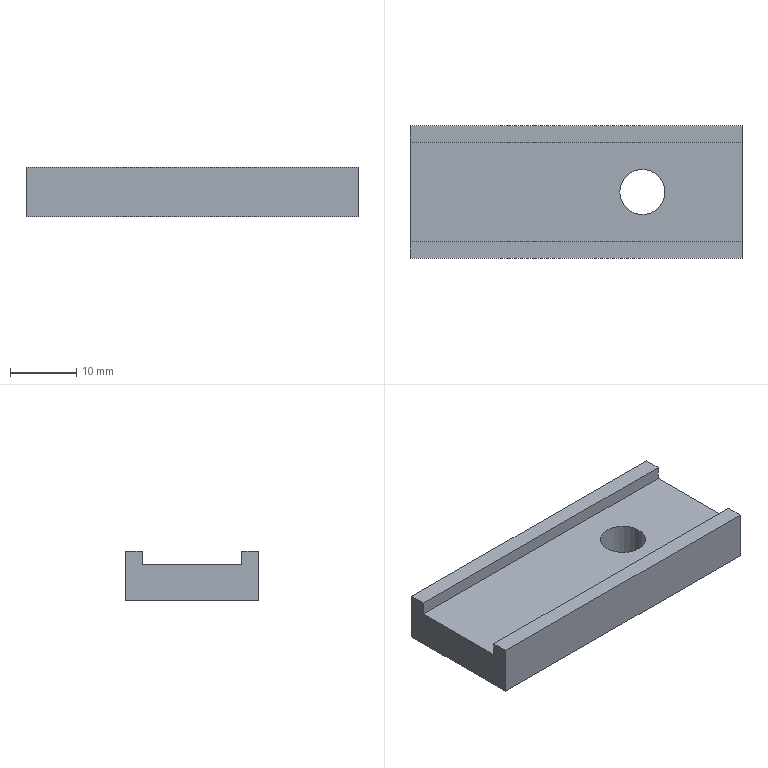Part | STEP file | Driven lead screw fixed block QY-1-17 | 1 solid | 12 faces | box 50 x 20 x 7.5 mm | volume 5800 mm3 | plane 10 | cylinder 2 | commonest cylinder face diameters 6.8 x2
STEP:
#1=CARTESIAN_POINT('',(0.,0.,0.));
#2=DIRECTION('',(0.,0.,1.));
#3=DIRECTION('',(1.,0.,0.));
#4=AXIS2_PLACEMENT_3D('',#1,#2,#3);
#5=CARTESIAN_POINT('',(13.4,0.,0.));
#6=VERTEX_POINT('',#5);
#7=CARTESIAN_POINT('',(13.4,0.,5.5));
#8=VERTEX_POINT('',#7);
#9=CARTESIAN_POINT('',(13.4,0.,5.5));
#10=DIRECTION('',(0.,0.,1.));
#11=VECTOR('',#10,1.);
#12=LINE('',#9,#11);
#13=CARTESIAN_POINT('',(10.,0.,5.5));
#14=DIRECTION('',(0.,0.,1.));
#15=DIRECTION('',(1.,0.,0.));
#16=AXIS2_PLACEMENT_3D('',#13,#14,#15);
#17=CYLINDRICAL_SURFACE('',#16,3.4);
#18=CARTESIAN_POINT('',(6.283,0.));
#19=DIRECTION('',(0.,1.));
#20=VECTOR('',#19,1.);
#21=LINE('',#18,#20);
#22=(GEOMETRIC_REPRESENTATION_CONTEXT(2)PARAMETRIC_REPRESENTATION_CONTEXT()REPRESENTATION_CONTEXT('',''));
#23=DEFINITIONAL_REPRESENTATION('',(#21),#22);
#24=PCURVE('',#17,#23);
#25=CARTESIAN_POINT('',(10.,0.,5.5));
#26=DIRECTION('',(0.,0.,1.));
#27=DIRECTION('',(1.,0.,0.));
#28=AXIS2_PLACEMENT_3D('',#25,#26,#27);
#29=CYLINDRICAL_SURFACE('',#28,3.4);
#30=CARTESIAN_POINT('',(0.,0.));
#31=DIRECTION('',(0.,1.));
#32=VECTOR('',#31,1.);
#33=LINE('',#30,#32);
#34=(GEOMETRIC_REPRESENTATION_CONTEXT(2)PARAMETRIC_REPRESENTATION_CONTEXT()REPRESENTATION_CONTEXT('',''));
#35=DEFINITIONAL_REPRESENTATION('',(#33),#34);
#36=PCURVE('',#29,#35);
#37=SURFACE_CURVE('',#12,(#24,#36),.PCURVE_S1.);
#38=EDGE_CURVE('',#6,#8,#37,.T.);
#39=ORIENTED_EDGE('',*,*,#38,.T.);
#40=CARTESIAN_POINT('',(6.6,0.,5.5));
#41=VERTEX_POINT('',#40);
#42=CARTESIAN_POINT('',(10.,0.,5.5));
#43=DIRECTION('',(0.,0.,1.));
#44=DIRECTION('',(1.,0.,0.));
#45=AXIS2_PLACEMENT_3D('',#42,#43,#44);
#46=CIRCLE('',#45,3.4);
#47=CARTESIAN_POINT('',(0.,0.));
#48=DIRECTION('',(1.,0.));
#49=VECTOR('',#48,1.);
#50=LINE('',#47,#49);
#51=(GEOMETRIC_REPRESENTATION_CONTEXT(2)PARAMETRIC_REPRESENTATION_CONTEXT()REPRESENTATION_CONTEXT('',''));
#52=DEFINITIONAL_REPRESENTATION('',(#50),#51);
#53=PCURVE('',#17,#52);
#54=CARTESIAN_POINT('',(0.,0.,5.5));
#55=DIRECTION('',(0.,0.,-1.));
#56=DIRECTION('',(-1.,0.,0.));
#57=AXIS2_PLACEMENT_3D('',#54,#55,#56);
#58=PLANE('',#57);
#59=CARTESIAN_POINT('',(-13.4,0.));
#60=CARTESIAN_POINT('',(-13.4,5.889));
#61=CARTESIAN_POINT('',(-8.3,2.944));
#62=CARTESIAN_POINT('',(-3.2,0.));
#63=CARTESIAN_POINT('',(-8.3,-2.944));
#64=CARTESIAN_POINT('',(-13.4,-5.889));
#65=CARTESIAN_POINT('',(-13.4,0.));
#66=(BOUNDED_CURVE()B_SPLINE_CURVE(2,(#59,#60,#61,#62,#63,#64,#65),.UNSPECIFIED.,.T.,.F.)B_SPLINE_CURVE_WITH_KNOTS((1,2,2,2,2,1),(-2.094,0.,2.094,4.189,6.283,8.378),.UNSPECIFIED.)CURVE()GEOMETRIC_REPRESENTATION_ITEM()RATIONAL_B_SPLINE_CURVE((1.,0.5,1.,0.5,1.,0.5,1.))REPRESENTATION_ITEM(''));
#67=(GEOMETRIC_REPRESENTATION_CONTEXT(2)PARAMETRIC_REPRESENTATION_CONTEXT()REPRESENTATION_CONTEXT('',''));
#68=DEFINITIONAL_REPRESENTATION('',(#66),#67);
#69=PCURVE('',#58,#68);
#70=SURFACE_CURVE('',#46,(#53,#69),.PCURVE_S1.);
#71=EDGE_CURVE('',#41,#8,#70,.T.);
#72=ORIENTED_EDGE('',*,*,#71,.F.);
#73=CARTESIAN_POINT('',(6.6,0.,0.));
#74=VERTEX_POINT('',#73);
#75=CARTESIAN_POINT('',(6.6,0.,5.5));
#76=DIRECTION('',(0.,0.,1.));
#77=VECTOR('',#76,1.);
#78=LINE('',#75,#77);
#79=CARTESIAN_POINT('',(3.142,0.));
#80=DIRECTION('',(0.,1.));
#81=VECTOR('',#80,1.);
#82=LINE('',#79,#81);
#83=(GEOMETRIC_REPRESENTATION_CONTEXT(2)PARAMETRIC_REPRESENTATION_CONTEXT()REPRESENTATION_CONTEXT('',''));
#84=DEFINITIONAL_REPRESENTATION('',(#82),#83);
#85=PCURVE('',#17,#84);
#86=CARTESIAN_POINT('',(3.142,0.));
#87=DIRECTION('',(0.,1.));
#88=VECTOR('',#87,1.);
#89=LINE('',#86,#88);
#90=(GEOMETRIC_REPRESENTATION_CONTEXT(2)PARAMETRIC_REPRESENTATION_CONTEXT()REPRESENTATION_CONTEXT('',''));
#91=DEFINITIONAL_REPRESENTATION('',(#89),#90);
#92=PCURVE('',#29,#91);
#93=SURFACE_CURVE('',#78,(#85,#92),.PCURVE_S1.);
#94=EDGE_CURVE('',#74,#41,#93,.T.);
#95=ORIENTED_EDGE('',*,*,#94,.F.);
#96=CARTESIAN_POINT('',(10.,0.,0.));
#97=DIRECTION('',(0.,0.,1.));
#98=DIRECTION('',(1.,0.,0.));
#99=AXIS2_PLACEMENT_3D('',#96,#97,#98);
#100=CIRCLE('',#99,3.4);
#101=CARTESIAN_POINT('',(0.,-5.5));
#102=DIRECTION('',(1.,0.));
#103=VECTOR('',#102,1.);
#104=LINE('',#101,#103);
#105=(GEOMETRIC_REPRESENTATION_CONTEXT(2)PARAMETRIC_REPRESENTATION_CONTEXT()REPRESENTATION_CONTEXT('',''));
#106=DEFINITIONAL_REPRESENTATION('',(#104),#105);
#107=PCURVE('',#17,#106);
#108=CARTESIAN_POINT('',(0.,0.,0.));
#109=DIRECTION('',(0.,0.,1.));
#110=DIRECTION('',(1.,0.,0.));
#111=AXIS2_PLACEMENT_3D('',#108,#109,#110);
#112=PLANE('',#111);
#113=CARTESIAN_POINT('',(10.,0.));
#114=DIRECTION('',(1.,0.));
#115=AXIS2_PLACEMENT_2D('',#113,#114);
#116=CIRCLE('',#115,3.4);
#117=(GEOMETRIC_REPRESENTATION_CONTEXT(2)PARAMETRIC_REPRESENTATION_CONTEXT()REPRESENTATION_CONTEXT('',''));
#118=DEFINITIONAL_REPRESENTATION('',(#116),#117);
#119=PCURVE('',#112,#118);
#120=SURFACE_CURVE('',#100,(#107,#119),.PCURVE_S1.);
#121=EDGE_CURVE('',#74,#6,#120,.T.);
#122=ORIENTED_EDGE('',*,*,#121,.T.);
#123=EDGE_LOOP('',(#39,#72,#95,#122));
#124=FACE_BOUND('',#123,.F.);
#125=ADVANCED_FACE('',(#124),#17,.F.);
#126=CARTESIAN_POINT('',(-25.,-7.5,7.5));
#127=VERTEX_POINT('',#126);
#128=CARTESIAN_POINT('',(25.,-7.5,7.5));
#129=VERTEX_POINT('',#128);
#130=CARTESIAN_POINT('',(0.,-7.5,7.5));
#131=DIRECTION('',(1.,0.,0.));
#132=VECTOR('',#131,1.);
#133=LINE('',#130,#132);
#134=CARTESIAN_POINT('',(0.,0.,7.5));
#135=DIRECTION('',(0.,0.,1.));
#136=DIRECTION('',(1.,0.,0.));
#137=AXIS2_PLACEMENT_3D('',#134,#135,#136);
#138=PLANE('',#137);
#139=CARTESIAN_POINT('',(0.,-7.5));
#140=DIRECTION('',(1.,0.));
#141=VECTOR('',#140,1.);
#142=LINE('',#139,#141);
#143=(GEOMETRIC_REPRESENTATION_CONTEXT(2)PARAMETRIC_REPRESENTATION_CONTEXT()REPRESENTATION_CONTEXT('',''));
#144=DEFINITIONAL_REPRESENTATION('',(#142),#143);
#145=PCURVE('',#138,#144);
#146=CARTESIAN_POINT('',(-35.049,-7.5,5.5));
#147=DIRECTION('',(0.,-1.,0.));
#148=DIRECTION('',(0.,0.,-1.));
#149=AXIS2_PLACEMENT_3D('',#146,#147,#148);
#150=PLANE('',#149);
#151=CARTESIAN_POINT('',(-2.,35.049));
#152=DIRECTION('',(0.,1.));
#153=VECTOR('',#152,1.);
#154=LINE('',#151,#153);
#155=(GEOMETRIC_REPRESENTATION_CONTEXT(2)PARAMETRIC_REPRESENTATION_CONTEXT()REPRESENTATION_CONTEXT('',''));
#156=DEFINITIONAL_REPRESENTATION('',(#154),#155);
#157=PCURVE('',#150,#156);
#158=SURFACE_CURVE('',#133,(#145,#157),.PCURVE_S1.);
#159=EDGE_CURVE('',#127,#129,#158,.T.);
#160=ORIENTED_EDGE('',*,*,#159,.F.);
#161=CARTESIAN_POINT('',(-25.,-10.,7.5));
#162=VERTEX_POINT('',#161);
#163=CARTESIAN_POINT('',(-25.,10.,7.5));
#164=DIRECTION('',(0.,-1.,0.));
#165=VECTOR('',#164,1.);
#166=LINE('',#163,#165);
#167=CARTESIAN_POINT('',(-25.,10.));
#168=DIRECTION('',(0.,-1.));
#169=VECTOR('',#168,1.);
#170=LINE('',#167,#169);
#171=(GEOMETRIC_REPRESENTATION_CONTEXT(2)PARAMETRIC_REPRESENTATION_CONTEXT()REPRESENTATION_CONTEXT('',''));
#172=DEFINITIONAL_REPRESENTATION('',(#170),#171);
#173=PCURVE('',#138,#172);
#174=CARTESIAN_POINT('',(-25.,10.,7.5));
#175=DIRECTION('',(1.,0.,0.));
#176=DIRECTION('',(0.,0.,-1.));
#177=AXIS2_PLACEMENT_3D('',#174,#175,#176);
#178=PLANE('',#177);
#179=CARTESIAN_POINT('',(0.,0.));
#180=DIRECTION('',(0.,-1.));
#181=VECTOR('',#180,1.);
#182=LINE('',#179,#181);
#183=(GEOMETRIC_REPRESENTATION_CONTEXT(2)PARAMETRIC_REPRESENTATION_CONTEXT()REPRESENTATION_CONTEXT('',''));
#184=DEFINITIONAL_REPRESENTATION('',(#182),#183);
#185=PCURVE('',#178,#184);
#186=SURFACE_CURVE('',#166,(#173,#185),.PCURVE_S1.);
#187=EDGE_CURVE('',#127,#162,#186,.T.);
#188=ORIENTED_EDGE('',*,*,#187,.T.);
#189=CARTESIAN_POINT('',(25.,-10.,7.5));
#190=VERTEX_POINT('',#189);
#191=CARTESIAN_POINT('',(-25.,-10.,7.5));
#192=DIRECTION('',(1.,0.,0.));
#193=VECTOR('',#192,1.);
#194=LINE('',#191,#193);
#195=CARTESIAN_POINT('',(-25.,-10.));
#196=DIRECTION('',(1.,0.));
#197=VECTOR('',#196,1.);
#198=LINE('',#195,#197);
#199=(GEOMETRIC_REPRESENTATION_CONTEXT(2)PARAMETRIC_REPRESENTATION_CONTEXT()REPRESENTATION_CONTEXT('',''));
#200=DEFINITIONAL_REPRESENTATION('',(#198),#199);
#201=PCURVE('',#138,#200);
#202=CARTESIAN_POINT('',(-25.,-10.,7.5));
#203=DIRECTION('',(0.,1.,0.));
#204=DIRECTION('',(0.,0.,1.));
#205=AXIS2_PLACEMENT_3D('',#202,#203,#204);
#206=PLANE('',#205);
#207=CARTESIAN_POINT('',(0.,0.));
#208=DIRECTION('',(0.,1.));
#209=VECTOR('',#208,1.);
#210=LINE('',#207,#209);
#211=(GEOMETRIC_REPRESENTATION_CONTEXT(2)PARAMETRIC_REPRESENTATION_CONTEXT()REPRESENTATION_CONTEXT('',''));
#212=DEFINITIONAL_REPRESENTATION('',(#210),#211);
#213=PCURVE('',#206,#212);
#214=SURFACE_CURVE('',#194,(#201,#213),.PCURVE_S1.);
#215=EDGE_CURVE('',#162,#190,#214,.T.);
#216=ORIENTED_EDGE('',*,*,#215,.T.);
#217=CARTESIAN_POINT('',(25.,10.,7.5));
#218=DIRECTION('',(0.,1.,0.));
#219=VECTOR('',#218,1.);
#220=LINE('',#217,#219);
#221=CARTESIAN_POINT('',(25.,10.));
#222=DIRECTION('',(0.,1.));
#223=VECTOR('',#222,1.);
#224=LINE('',#221,#223);
#225=(GEOMETRIC_REPRESENTATION_CONTEXT(2)PARAMETRIC_REPRESENTATION_CONTEXT()REPRESENTATION_CONTEXT('',''));
#226=DEFINITIONAL_REPRESENTATION('',(#224),#225);
#227=PCURVE('',#138,#226);
#228=CARTESIAN_POINT('',(25.,10.,7.5));
#229=DIRECTION('',(-1.,0.,0.));
#230=DIRECTION('',(0.,-1.,0.));
#231=AXIS2_PLACEMENT_3D('',#228,#229,#230);
#232=PLANE('',#231);
#233=CARTESIAN_POINT('',(0.,0.));
#234=DIRECTION('',(-1.,0.));
#235=VECTOR('',#234,1.);
#236=LINE('',#233,#235);
#237=(GEOMETRIC_REPRESENTATION_CONTEXT(2)PARAMETRIC_REPRESENTATION_CONTEXT()REPRESENTATION_CONTEXT('',''));
#238=DEFINITIONAL_REPRESENTATION('',(#236),#237);
#239=PCURVE('',#232,#238);
#240=SURFACE_CURVE('',#220,(#227,#239),.PCURVE_S1.);
#241=EDGE_CURVE('',#190,#129,#240,.T.);
#242=ORIENTED_EDGE('',*,*,#241,.T.);
#243=EDGE_LOOP('',(#160,#188,#216,#242));
#244=FACE_BOUND('',#243,.T.);
#245=ADVANCED_FACE('',(#244),#138,.T.);
#246=CARTESIAN_POINT('',(25.,7.5,5.5));
#247=VERTEX_POINT('',#246);
#248=CARTESIAN_POINT('',(25.,-7.5,5.5));
#249=VERTEX_POINT('',#248);
#250=CARTESIAN_POINT('',(25.,10.,5.5));
#251=DIRECTION('',(0.,-1.,0.));
#252=VECTOR('',#251,1.);
#253=LINE('',#250,#252);
#254=CARTESIAN_POINT('',(0.,-2.));
#255=DIRECTION('',(1.,0.));
#256=VECTOR('',#255,1.);
#257=LINE('',#254,#256);
#258=(GEOMETRIC_REPRESENTATION_CONTEXT(2)PARAMETRIC_REPRESENTATION_CONTEXT()REPRESENTATION_CONTEXT('',''));
#259=DEFINITIONAL_REPRESENTATION('',(#257),#258);
#260=PCURVE('',#232,#259);
#261=CARTESIAN_POINT('',(-25.,10.));
#262=DIRECTION('',(0.,-1.));
#263=VECTOR('',#262,1.);
#264=LINE('',#261,#263);
#265=(GEOMETRIC_REPRESENTATION_CONTEXT(2)PARAMETRIC_REPRESENTATION_CONTEXT()REPRESENTATION_CONTEXT('',''));
#266=DEFINITIONAL_REPRESENTATION('',(#264),#265);
#267=PCURVE('',#58,#266);
#268=SURFACE_CURVE('',#253,(#260,#267),.PCURVE_S1.);
#269=EDGE_CURVE('',#247,#249,#268,.T.);
#270=ORIENTED_EDGE('',*,*,#269,.T.);
#271=CARTESIAN_POINT('',(25.,-7.5,7.5));
#272=DIRECTION('',(0.,0.,1.));
#273=VECTOR('',#272,1.);
#274=LINE('',#271,#273);
#275=CARTESIAN_POINT('',(17.5,0.));
#276=DIRECTION('',(0.,1.));
#277=VECTOR('',#276,1.);
#278=LINE('',#275,#277);
#279=(GEOMETRIC_REPRESENTATION_CONTEXT(2)PARAMETRIC_REPRESENTATION_CONTEXT()REPRESENTATION_CONTEXT('',''));
#280=DEFINITIONAL_REPRESENTATION('',(#278),#279);
#281=PCURVE('',#232,#280);
#282=CARTESIAN_POINT('',(-2.,60.049));
#283=DIRECTION('',(-1.,0.));
#284=VECTOR('',#283,1.);
#285=LINE('',#282,#284);
#286=(GEOMETRIC_REPRESENTATION_CONTEXT(2)PARAMETRIC_REPRESENTATION_CONTEXT()REPRESENTATION_CONTEXT('',''));
#287=DEFINITIONAL_REPRESENTATION('',(#285),#286);
#288=PCURVE('',#150,#287);
#289=SURFACE_CURVE('',#274,(#281,#288),.PCURVE_S1.);
#290=EDGE_CURVE('',#249,#129,#289,.T.);
#291=ORIENTED_EDGE('',*,*,#290,.T.);
#292=ORIENTED_EDGE('',*,*,#241,.F.);
#293=CARTESIAN_POINT('',(25.,-10.,0.));
#294=VERTEX_POINT('',#293);
#295=CARTESIAN_POINT('',(25.,-10.,7.5));
#296=DIRECTION('',(0.,0.,-1.));
#297=VECTOR('',#296,1.);
#298=LINE('',#295,#297);
#299=CARTESIAN_POINT('',(20.,0.));
#300=DIRECTION('',(0.,-1.));
#301=VECTOR('',#300,1.);
#302=LINE('',#299,#301);
#303=(GEOMETRIC_REPRESENTATION_CONTEXT(2)PARAMETRIC_REPRESENTATION_CONTEXT()REPRESENTATION_CONTEXT('',''));
#304=DEFINITIONAL_REPRESENTATION('',(#302),#303);
#305=PCURVE('',#232,#304);
#306=CARTESIAN_POINT('',(0.,50.));
#307=DIRECTION('',(-1.,0.));
#308=VECTOR('',#307,1.);
#309=LINE('',#306,#308);
#310=(GEOMETRIC_REPRESENTATION_CONTEXT(2)PARAMETRIC_REPRESENTATION_CONTEXT()REPRESENTATION_CONTEXT('',''));
#311=DEFINITIONAL_REPRESENTATION('',(#309),#310);
#312=PCURVE('',#206,#311);
#313=SURFACE_CURVE('',#298,(#305,#312),.PCURVE_S1.);
#314=EDGE_CURVE('',#190,#294,#313,.T.);
#315=ORIENTED_EDGE('',*,*,#314,.T.);
#316=CARTESIAN_POINT('',(25.,10.,0.));
#317=VERTEX_POINT('',#316);
#318=CARTESIAN_POINT('',(25.,10.,0.));
#319=DIRECTION('',(0.,1.,0.));
#320=VECTOR('',#319,1.);
#321=LINE('',#318,#320);
#322=CARTESIAN_POINT('',(0.,-7.5));
#323=DIRECTION('',(-1.,0.));
#324=VECTOR('',#323,1.);
#325=LINE('',#322,#324);
#326=(GEOMETRIC_REPRESENTATION_CONTEXT(2)PARAMETRIC_REPRESENTATION_CONTEXT()REPRESENTATION_CONTEXT('',''));
#327=DEFINITIONAL_REPRESENTATION('',(#325),#326);
#328=PCURVE('',#232,#327);
#329=CARTESIAN_POINT('',(25.,10.));
#330=DIRECTION('',(0.,1.));
#331=VECTOR('',#330,1.);
#332=LINE('',#329,#331);
#333=(GEOMETRIC_REPRESENTATION_CONTEXT(2)PARAMETRIC_REPRESENTATION_CONTEXT()REPRESENTATION_CONTEXT('',''));
#334=DEFINITIONAL_REPRESENTATION('',(#332),#333);
#335=PCURVE('',#112,#334);
#336=SURFACE_CURVE('',#321,(#328,#335),.PCURVE_S1.);
#337=EDGE_CURVE('',#294,#317,#336,.T.);
#338=ORIENTED_EDGE('',*,*,#337,.T.);
#339=CARTESIAN_POINT('',(25.,10.,7.5));
#340=VERTEX_POINT('',#339);
#341=CARTESIAN_POINT('',(25.,10.,7.5));
#342=DIRECTION('',(0.,0.,-1.));
#343=VECTOR('',#342,1.);
#344=LINE('',#341,#343);
#345=CARTESIAN_POINT('',(0.,0.));
#346=DIRECTION('',(0.,-1.));
#347=VECTOR('',#346,1.);
#348=LINE('',#345,#347);
#349=(GEOMETRIC_REPRESENTATION_CONTEXT(2)PARAMETRIC_REPRESENTATION_CONTEXT()REPRESENTATION_CONTEXT('',''));
#350=DEFINITIONAL_REPRESENTATION('',(#348),#349);
#351=PCURVE('',#232,#350);
#352=CARTESIAN_POINT('',(-25.,10.,7.5));
#353=DIRECTION('',(0.,-1.,0.));
#354=DIRECTION('',(0.,0.,-1.));
#355=AXIS2_PLACEMENT_3D('',#352,#353,#354);
#356=PLANE('',#355);
#357=CARTESIAN_POINT('',(0.,50.));
#358=DIRECTION('',(1.,0.));
#359=VECTOR('',#358,1.);
#360=LINE('',#357,#359);
#361=(GEOMETRIC_REPRESENTATION_CONTEXT(2)PARAMETRIC_REPRESENTATION_CONTEXT()REPRESENTATION_CONTEXT('',''));
#362=DEFINITIONAL_REPRESENTATION('',(#360),#361);
#363=PCURVE('',#356,#362);
#364=SURFACE_CURVE('',#344,(#351,#363),.PCURVE_S1.);
#365=EDGE_CURVE('',#340,#317,#364,.T.);
#366=ORIENTED_EDGE('',*,*,#365,.F.);
#367=CARTESIAN_POINT('',(25.,7.5,7.5));
#368=VERTEX_POINT('',#367);
#369=CARTESIAN_POINT('',(25.,10.,7.5));
#370=DIRECTION('',(0.,1.,0.));
#371=VECTOR('',#370,1.);
#372=LINE('',#369,#371);
#373=CARTESIAN_POINT('',(0.,0.));
#374=DIRECTION('',(-1.,0.));
#375=VECTOR('',#374,1.);
#376=LINE('',#373,#375);
#377=(GEOMETRIC_REPRESENTATION_CONTEXT(2)PARAMETRIC_REPRESENTATION_CONTEXT()REPRESENTATION_CONTEXT('',''));
#378=DEFINITIONAL_REPRESENTATION('',(#376),#377);
#379=PCURVE('',#232,#378);
#380=CARTESIAN_POINT('',(0.,0.,7.5));
#381=DIRECTION('',(0.,0.,1.));
#382=DIRECTION('',(1.,0.,0.));
#383=AXIS2_PLACEMENT_3D('',#380,#381,#382);
#384=PLANE('',#383);
#385=CARTESIAN_POINT('',(25.,10.));
#386=DIRECTION('',(0.,1.));
#387=VECTOR('',#386,1.);
#388=LINE('',#385,#387);
#389=(GEOMETRIC_REPRESENTATION_CONTEXT(2)PARAMETRIC_REPRESENTATION_CONTEXT()REPRESENTATION_CONTEXT('',''));
#390=DEFINITIONAL_REPRESENTATION('',(#388),#389);
#391=PCURVE('',#384,#390);
#392=SURFACE_CURVE('',#372,(#379,#391),.PCURVE_S1.);
#393=EDGE_CURVE('',#368,#340,#392,.T.);
#394=ORIENTED_EDGE('',*,*,#393,.F.);
#395=CARTESIAN_POINT('',(25.,7.5,7.5));
#396=DIRECTION('',(0.,0.,-1.));
#397=VECTOR('',#396,1.);
#398=LINE('',#395,#397);
#399=CARTESIAN_POINT('',(2.5,0.));
#400=DIRECTION('',(0.,-1.));
#401=VECTOR('',#400,1.);
#402=LINE('',#399,#401);
#403=(GEOMETRIC_REPRESENTATION_CONTEXT(2)PARAMETRIC_REPRESENTATION_CONTEXT()REPRESENTATION_CONTEXT('',''));
#404=DEFINITIONAL_REPRESENTATION('',(#402),#403);
#405=PCURVE('',#232,#404);
#406=CARTESIAN_POINT('',(-35.049,7.5,5.5));
#407=DIRECTION('',(0.,1.,0.));
#408=DIRECTION('',(0.,0.,1.));
#409=AXIS2_PLACEMENT_3D('',#406,#407,#408);
#410=PLANE('',#409);
#411=CARTESIAN_POINT('',(2.,60.049));
#412=DIRECTION('',(-1.,0.));
#413=VECTOR('',#412,1.);
#414=LINE('',#411,#413);
#415=(GEOMETRIC_REPRESENTATION_CONTEXT(2)PARAMETRIC_REPRESENTATION_CONTEXT()REPRESENTATION_CONTEXT('',''));
#416=DEFINITIONAL_REPRESENTATION('',(#414),#415);
#417=PCURVE('',#410,#416);
#418=SURFACE_CURVE('',#398,(#405,#417),.PCURVE_S1.);
#419=EDGE_CURVE('',#368,#247,#418,.T.);
#420=ORIENTED_EDGE('',*,*,#419,.T.);
#421=EDGE_LOOP('',(#270,#291,#292,#315,#338,#366,#394,#420));
#422=FACE_BOUND('',#421,.T.);
#423=ADVANCED_FACE('',(#422),#232,.F.);
#424=CARTESIAN_POINT('',(-25.,10.,0.));
#425=VERTEX_POINT('',#424);
#426=CARTESIAN_POINT('',(-25.,10.,0.));
#427=DIRECTION('',(-1.,0.,0.));
#428=VECTOR('',#427,1.);
#429=LINE('',#426,#428);
#430=CARTESIAN_POINT('',(7.5,0.));
#431=DIRECTION('',(0.,-1.));
#432=VECTOR('',#431,1.);
#433=LINE('',#430,#432);
#434=(GEOMETRIC_REPRESENTATION_CONTEXT(2)PARAMETRIC_REPRESENTATION_CONTEXT()REPRESENTATION_CONTEXT('',''));
#435=DEFINITIONAL_REPRESENTATION('',(#433),#434);
#436=PCURVE('',#356,#435);
#437=CARTESIAN_POINT('',(-25.,10.));
#438=DIRECTION('',(-1.,0.));
#439=VECTOR('',#438,1.);
#440=LINE('',#437,#439);
#441=(GEOMETRIC_REPRESENTATION_CONTEXT(2)PARAMETRIC_REPRESENTATION_CONTEXT()REPRESENTATION_CONTEXT('',''));
#442=DEFINITIONAL_REPRESENTATION('',(#440),#441);
#443=PCURVE('',#112,#442);
#444=SURFACE_CURVE('',#429,(#436,#443),.PCURVE_S1.);
#445=EDGE_CURVE('',#317,#425,#444,.T.);
#446=ORIENTED_EDGE('',*,*,#445,.T.);
#447=CARTESIAN_POINT('',(-25.,10.,7.5));
#448=VERTEX_POINT('',#447);
#449=CARTESIAN_POINT('',(-25.,10.,7.5));
#450=DIRECTION('',(0.,0.,-1.));
#451=VECTOR('',#450,1.);
#452=LINE('',#449,#451);
#453=CARTESIAN_POINT('',(0.,0.));
#454=DIRECTION('',(1.,0.));
#455=VECTOR('',#454,1.);
#456=LINE('',#453,#455);
#457=(GEOMETRIC_REPRESENTATION_CONTEXT(2)PARAMETRIC_REPRESENTATION_CONTEXT()REPRESENTATION_CONTEXT('',''));
#458=DEFINITIONAL_REPRESENTATION('',(#456),#457);
#459=PCURVE('',#356,#458);
#460=CARTESIAN_POINT('',(0.,0.));
#461=DIRECTION('',(1.,0.));
#462=VECTOR('',#461,1.);
#463=LINE('',#460,#462);
#464=(GEOMETRIC_REPRESENTATION_CONTEXT(2)PARAMETRIC_REPRESENTATION_CONTEXT()REPRESENTATION_CONTEXT('',''));
#465=DEFINITIONAL_REPRESENTATION('',(#463),#464);
#466=PCURVE('',#178,#465);
#467=SURFACE_CURVE('',#452,(#459,#466),.PCURVE_S1.);
#468=EDGE_CURVE('',#448,#425,#467,.T.);
#469=ORIENTED_EDGE('',*,*,#468,.F.);
#470=CARTESIAN_POINT('',(-25.,10.,7.5));
#471=DIRECTION('',(-1.,0.,0.));
#472=VECTOR('',#471,1.);
#473=LINE('',#470,#472);
#474=CARTESIAN_POINT('',(0.,0.));
#475=DIRECTION('',(0.,-1.));
#476=VECTOR('',#475,1.);
#477=LINE('',#474,#476);
#478=(GEOMETRIC_REPRESENTATION_CONTEXT(2)PARAMETRIC_REPRESENTATION_CONTEXT()REPRESENTATION_CONTEXT('',''));
#479=DEFINITIONAL_REPRESENTATION('',(#477),#478);
#480=PCURVE('',#356,#479);
#481=CARTESIAN_POINT('',(-25.,10.));
#482=DIRECTION('',(-1.,0.));
#483=VECTOR('',#482,1.);
#484=LINE('',#481,#483);
#485=(GEOMETRIC_REPRESENTATION_CONTEXT(2)PARAMETRIC_REPRESENTATION_CONTEXT()REPRESENTATION_CONTEXT('',''));
#486=DEFINITIONAL_REPRESENTATION('',(#484),#485);
#487=PCURVE('',#384,#486);
#488=SURFACE_CURVE('',#473,(#480,#487),.PCURVE_S1.);
#489=EDGE_CURVE('',#340,#448,#488,.T.);
#490=ORIENTED_EDGE('',*,*,#489,.F.);
#491=ORIENTED_EDGE('',*,*,#365,.T.);
#492=EDGE_LOOP('',(#446,#469,#490,#491));
#493=FACE_BOUND('',#492,.T.);
#494=ADVANCED_FACE('',(#493),#356,.F.);
#495=ORIENTED_EDGE('',*,*,#187,.F.);
#496=CARTESIAN_POINT('',(-25.,-7.5,5.5));
#497=VERTEX_POINT('',#496);
#498=CARTESIAN_POINT('',(-25.,-7.5,7.5));
#499=DIRECTION('',(0.,0.,-1.));
#500=VECTOR('',#499,1.);
#501=LINE('',#498,#500);
#502=CARTESIAN_POINT('',(0.,-17.5));
#503=DIRECTION('',(1.,0.));
#504=VECTOR('',#503,1.);
#505=LINE('',#502,#504);
#506=(GEOMETRIC_REPRESENTATION_CONTEXT(2)PARAMETRIC_REPRESENTATION_CONTEXT()REPRESENTATION_CONTEXT('',''));
#507=DEFINITIONAL_REPRESENTATION('',(#505),#506);
#508=PCURVE('',#178,#507);
#509=CARTESIAN_POINT('',(-2.,10.049));
#510=DIRECTION('',(1.,0.));
#511=VECTOR('',#510,1.);
#512=LINE('',#509,#511);
#513=(GEOMETRIC_REPRESENTATION_CONTEXT(2)PARAMETRIC_REPRESENTATION_CONTEXT()REPRESENTATION_CONTEXT('',''));
#514=DEFINITIONAL_REPRESENTATION('',(#512),#513);
#515=PCURVE('',#150,#514);
#516=SURFACE_CURVE('',#501,(#508,#515),.PCURVE_S1.);
#517=EDGE_CURVE('',#127,#497,#516,.T.);
#518=ORIENTED_EDGE('',*,*,#517,.T.);
#519=CARTESIAN_POINT('',(-25.,7.5,5.5));
#520=VERTEX_POINT('',#519);
#521=CARTESIAN_POINT('',(-25.,10.,5.5));
#522=DIRECTION('',(0.,1.,0.));
#523=VECTOR('',#522,1.);
#524=LINE('',#521,#523);
#525=CARTESIAN_POINT('',(2.,0.));
#526=DIRECTION('',(0.,1.));
#527=VECTOR('',#526,1.);
#528=LINE('',#525,#527);
#529=(GEOMETRIC_REPRESENTATION_CONTEXT(2)PARAMETRIC_REPRESENTATION_CONTEXT()REPRESENTATION_CONTEXT('',''));
#530=DEFINITIONAL_REPRESENTATION('',(#528),#529);
#531=PCURVE('',#178,#530);
#532=CARTESIAN_POINT('',(25.,10.));
#533=DIRECTION('',(0.,1.));
#534=VECTOR('',#533,1.);
#535=LINE('',#532,#534);
#536=(GEOMETRIC_REPRESENTATION_CONTEXT(2)PARAMETRIC_REPRESENTATION_CONTEXT()REPRESENTATION_CONTEXT('',''));
#537=DEFINITIONAL_REPRESENTATION('',(#535),#536);
#538=PCURVE('',#58,#537);
#539=SURFACE_CURVE('',#524,(#531,#538),.PCURVE_S1.);
#540=EDGE_CURVE('',#497,#520,#539,.T.);
#541=ORIENTED_EDGE('',*,*,#540,.T.);
#542=CARTESIAN_POINT('',(-25.,7.5,7.5));
#543=VERTEX_POINT('',#542);
#544=CARTESIAN_POINT('',(-25.,7.5,7.5));
#545=DIRECTION('',(0.,0.,1.));
#546=VECTOR('',#545,1.);
#547=LINE('',#544,#546);
#548=CARTESIAN_POINT('',(0.,-2.5));
#549=DIRECTION('',(-1.,0.));
#550=VECTOR('',#549,1.);
#551=LINE('',#548,#550);
#552=(GEOMETRIC_REPRESENTATION_CONTEXT(2)PARAMETRIC_REPRESENTATION_CONTEXT()REPRESENTATION_CONTEXT('',''));
#553=DEFINITIONAL_REPRESENTATION('',(#551),#552);
#554=PCURVE('',#178,#553);
#555=CARTESIAN_POINT('',(2.,10.049));
#556=DIRECTION('',(1.,0.));
#557=VECTOR('',#556,1.);
#558=LINE('',#555,#557);
#559=(GEOMETRIC_REPRESENTATION_CONTEXT(2)PARAMETRIC_REPRESENTATION_CONTEXT()REPRESENTATION_CONTEXT('',''));
#560=DEFINITIONAL_REPRESENTATION('',(#558),#559);
#561=PCURVE('',#410,#560);
#562=SURFACE_CURVE('',#547,(#554,#561),.PCURVE_S1.);
#563=EDGE_CURVE('',#520,#543,#562,.T.);
#564=ORIENTED_EDGE('',*,*,#563,.T.);
#565=CARTESIAN_POINT('',(-25.,10.,7.5));
#566=DIRECTION('',(0.,-1.,0.));
#567=VECTOR('',#566,1.);
#568=LINE('',#565,#567);
#569=CARTESIAN_POINT('',(0.,0.));
#570=DIRECTION('',(0.,-1.));
#571=VECTOR('',#570,1.);
#572=LINE('',#569,#571);
#573=(GEOMETRIC_REPRESENTATION_CONTEXT(2)PARAMETRIC_REPRESENTATION_CONTEXT()REPRESENTATION_CONTEXT('',''));
#574=DEFINITIONAL_REPRESENTATION('',(#572),#573);
#575=PCURVE('',#178,#574);
#576=CARTESIAN_POINT('',(-25.,10.));
#577=DIRECTION('',(0.,-1.));
#578=VECTOR('',#577,1.);
#579=LINE('',#576,#578);
#580=(GEOMETRIC_REPRESENTATION_CONTEXT(2)PARAMETRIC_REPRESENTATION_CONTEXT()REPRESENTATION_CONTEXT('',''));
#581=DEFINITIONAL_REPRESENTATION('',(#579),#580);
#582=PCURVE('',#384,#581);
#583=SURFACE_CURVE('',#568,(#575,#582),.PCURVE_S1.);
#584=EDGE_CURVE('',#448,#543,#583,.T.);
#585=ORIENTED_EDGE('',*,*,#584,.F.);
#586=ORIENTED_EDGE('',*,*,#468,.T.);
#587=CARTESIAN_POINT('',(-25.,-10.,0.));
#588=VERTEX_POINT('',#587);
#589=CARTESIAN_POINT('',(-25.,10.,0.));
#590=DIRECTION('',(0.,-1.,0.));
#591=VECTOR('',#590,1.);
#592=LINE('',#589,#591);
#593=CARTESIAN_POINT('',(7.5,0.));
#594=DIRECTION('',(0.,-1.));
#595=VECTOR('',#594,1.);
#596=LINE('',#593,#595);
#597=(GEOMETRIC_REPRESENTATION_CONTEXT(2)PARAMETRIC_REPRESENTATION_CONTEXT()REPRESENTATION_CONTEXT('',''));
#598=DEFINITIONAL_REPRESENTATION('',(#596),#597);
#599=PCURVE('',#178,#598);
#600=CARTESIAN_POINT('',(-25.,10.));
#601=DIRECTION('',(0.,-1.));
#602=VECTOR('',#601,1.);
#603=LINE('',#600,#602);
#604=(GEOMETRIC_REPRESENTATION_CONTEXT(2)PARAMETRIC_REPRESENTATION_CONTEXT()REPRESENTATION_CONTEXT('',''));
#605=DEFINITIONAL_REPRESENTATION('',(#603),#604);
#606=PCURVE('',#112,#605);
#607=SURFACE_CURVE('',#592,(#599,#606),.PCURVE_S1.);
#608=EDGE_CURVE('',#425,#588,#607,.T.);
#609=ORIENTED_EDGE('',*,*,#608,.T.);
#610=CARTESIAN_POINT('',(-25.,-10.,7.5));
#611=DIRECTION('',(0.,0.,-1.));
#612=VECTOR('',#611,1.);
#613=LINE('',#610,#612);
#614=CARTESIAN_POINT('',(0.,-20.));
#615=DIRECTION('',(1.,0.));
#616=VECTOR('',#615,1.);
#617=LINE('',#614,#616);
#618=(GEOMETRIC_REPRESENTATION_CONTEXT(2)PARAMETRIC_REPRESENTATION_CONTEXT()REPRESENTATION_CONTEXT('',''));
#619=DEFINITIONAL_REPRESENTATION('',(#617),#618);
#620=PCURVE('',#178,#619);
#621=CARTESIAN_POINT('',(0.,0.));
#622=DIRECTION('',(-1.,0.));
#623=VECTOR('',#622,1.);
#624=LINE('',#621,#623);
#625=(GEOMETRIC_REPRESENTATION_CONTEXT(2)PARAMETRIC_REPRESENTATION_CONTEXT()REPRESENTATION_CONTEXT('',''));
#626=DEFINITIONAL_REPRESENTATION('',(#624),#625);
#627=PCURVE('',#206,#626);
#628=SURFACE_CURVE('',#613,(#620,#627),.PCURVE_S1.);
#629=EDGE_CURVE('',#162,#588,#628,.T.);
#630=ORIENTED_EDGE('',*,*,#629,.F.);
#631=EDGE_LOOP('',(#495,#518,#541,#564,#585,#586,#609,#630));
#632=FACE_BOUND('',#631,.T.);
#633=ADVANCED_FACE('',(#632),#178,.F.);
#634=CARTESIAN_POINT('',(-25.,-10.,0.));
#635=DIRECTION('',(1.,0.,0.));
#636=VECTOR('',#635,1.);
#637=LINE('',#634,#636);
#638=CARTESIAN_POINT('',(-7.5,0.));
#639=DIRECTION('',(0.,1.));
#640=VECTOR('',#639,1.);
#641=LINE('',#638,#640);
#642=(GEOMETRIC_REPRESENTATION_CONTEXT(2)PARAMETRIC_REPRESENTATION_CONTEXT()REPRESENTATION_CONTEXT('',''));
#643=DEFINITIONAL_REPRESENTATION('',(#641),#642);
#644=PCURVE('',#206,#643);
#645=CARTESIAN_POINT('',(-25.,-10.));
#646=DIRECTION('',(1.,0.));
#647=VECTOR('',#646,1.);
#648=LINE('',#645,#647);
#649=(GEOMETRIC_REPRESENTATION_CONTEXT(2)PARAMETRIC_REPRESENTATION_CONTEXT()REPRESENTATION_CONTEXT('',''));
#650=DEFINITIONAL_REPRESENTATION('',(#648),#649);
#651=PCURVE('',#112,#650);
#652=SURFACE_CURVE('',#637,(#644,#651),.PCURVE_S1.);
#653=EDGE_CURVE('',#588,#294,#652,.T.);
#654=ORIENTED_EDGE('',*,*,#653,.T.);
#655=ORIENTED_EDGE('',*,*,#314,.F.);
#656=ORIENTED_EDGE('',*,*,#215,.F.);
#657=ORIENTED_EDGE('',*,*,#629,.T.);
#658=EDGE_LOOP('',(#654,#655,#656,#657));
#659=FACE_BOUND('',#658,.T.);
#660=ADVANCED_FACE('',(#659),#206,.F.);
#661=CARTESIAN_POINT('',(0.,7.5,7.5));
#662=DIRECTION('',(-1.,0.,0.));
#663=VECTOR('',#662,1.);
#664=LINE('',#661,#663);
#665=CARTESIAN_POINT('',(0.,7.5));
#666=DIRECTION('',(-1.,0.));
#667=VECTOR('',#666,1.);
#668=LINE('',#665,#667);
#669=(GEOMETRIC_REPRESENTATION_CONTEXT(2)PARAMETRIC_REPRESENTATION_CONTEXT()REPRESENTATION_CONTEXT('',''));
#670=DEFINITIONAL_REPRESENTATION('',(#668),#669);
#671=PCURVE('',#384,#670);
#672=CARTESIAN_POINT('',(2.,35.049));
#673=DIRECTION('',(0.,-1.));
#674=VECTOR('',#673,1.);
#675=LINE('',#672,#674);
#676=(GEOMETRIC_REPRESENTATION_CONTEXT(2)PARAMETRIC_REPRESENTATION_CONTEXT()REPRESENTATION_CONTEXT('',''));
#677=DEFINITIONAL_REPRESENTATION('',(#675),#676);
#678=PCURVE('',#410,#677);
#679=SURFACE_CURVE('',#664,(#671,#678),.PCURVE_S1.);
#680=EDGE_CURVE('',#368,#543,#679,.T.);
#681=ORIENTED_EDGE('',*,*,#680,.F.);
#682=ORIENTED_EDGE('',*,*,#393,.T.);
#683=ORIENTED_EDGE('',*,*,#489,.T.);
#684=ORIENTED_EDGE('',*,*,#584,.T.);
#685=EDGE_LOOP('',(#681,#682,#683,#684));
#686=FACE_BOUND('',#685,.T.);
#687=ADVANCED_FACE('',(#686),#384,.T.);
#688=CARTESIAN_POINT('',(10.,0.,0.));
#689=DIRECTION('',(0.,0.,1.));
#690=DIRECTION('',(1.,0.,0.));
#691=AXIS2_PLACEMENT_3D('',#688,#689,#690);
#692=CIRCLE('',#691,3.4);
#693=CARTESIAN_POINT('',(10.,0.));
#694=DIRECTION('',(1.,0.));
#695=AXIS2_PLACEMENT_2D('',#693,#694);
#696=CIRCLE('',#695,3.4);
#697=(GEOMETRIC_REPRESENTATION_CONTEXT(2)PARAMETRIC_REPRESENTATION_CONTEXT()REPRESENTATION_CONTEXT('',''));
#698=DEFINITIONAL_REPRESENTATION('',(#696),#697);
#699=PCURVE('',#112,#698);
#700=CARTESIAN_POINT('',(0.,-5.5));
#701=DIRECTION('',(1.,0.));
#702=VECTOR('',#701,1.);
#703=LINE('',#700,#702);
#704=(GEOMETRIC_REPRESENTATION_CONTEXT(2)PARAMETRIC_REPRESENTATION_CONTEXT()REPRESENTATION_CONTEXT('',''));
#705=DEFINITIONAL_REPRESENTATION('',(#703),#704);
#706=PCURVE('',#29,#705);
#707=SURFACE_CURVE('',#692,(#699,#706),.PCURVE_S1.);
#708=EDGE_CURVE('',#6,#74,#707,.T.);
#709=ORIENTED_EDGE('',*,*,#708,.T.);
#710=ORIENTED_EDGE('',*,*,#121,.T.);
#711=EDGE_LOOP('',(#709,#710));
#712=FACE_BOUND('',#711,.T.);
#713=ORIENTED_EDGE('',*,*,#337,.F.);
#714=ORIENTED_EDGE('',*,*,#653,.F.);
#715=ORIENTED_EDGE('',*,*,#608,.F.);
#716=ORIENTED_EDGE('',*,*,#445,.F.);
#717=EDGE_LOOP('',(#713,#714,#715,#716));
#718=FACE_BOUND('',#717,.T.);
#719=ADVANCED_FACE('',(#712,#718),#112,.F.);
#720=CARTESIAN_POINT('',(10.,0.,5.5));
#721=DIRECTION('',(0.,0.,1.));
#722=DIRECTION('',(1.,0.,0.));
#723=AXIS2_PLACEMENT_3D('',#720,#721,#722);
#724=CIRCLE('',#723,3.4);
#725=CARTESIAN_POINT('',(-13.4,0.));
#726=CARTESIAN_POINT('',(-13.4,5.889));
#727=CARTESIAN_POINT('',(-8.3,2.944));
#728=CARTESIAN_POINT('',(-3.2,0.));
#729=CARTESIAN_POINT('',(-8.3,-2.944));
#730=CARTESIAN_POINT('',(-13.4,-5.889));
#731=CARTESIAN_POINT('',(-13.4,0.));
#732=(BOUNDED_CURVE()B_SPLINE_CURVE(2,(#725,#726,#727,#728,#729,#730,#731),.UNSPECIFIED.,.T.,.F.)B_SPLINE_CURVE_WITH_KNOTS((1,2,2,2,2,1),(-2.094,0.,2.094,4.189,6.283,8.378),.UNSPECIFIED.)CURVE()GEOMETRIC_REPRESENTATION_ITEM()RATIONAL_B_SPLINE_CURVE((1.,0.5,1.,0.5,1.,0.5,1.))REPRESENTATION_ITEM(''));
#733=(GEOMETRIC_REPRESENTATION_CONTEXT(2)PARAMETRIC_REPRESENTATION_CONTEXT()REPRESENTATION_CONTEXT('',''));
#734=DEFINITIONAL_REPRESENTATION('',(#732),#733);
#735=PCURVE('',#58,#734);
#736=CARTESIAN_POINT('',(0.,0.));
#737=DIRECTION('',(1.,0.));
#738=VECTOR('',#737,1.);
#739=LINE('',#736,#738);
#740=(GEOMETRIC_REPRESENTATION_CONTEXT(2)PARAMETRIC_REPRESENTATION_CONTEXT()REPRESENTATION_CONTEXT('',''));
#741=DEFINITIONAL_REPRESENTATION('',(#739),#740);
#742=PCURVE('',#29,#741);
#743=SURFACE_CURVE('',#724,(#735,#742),.PCURVE_S1.);
#744=EDGE_CURVE('',#8,#41,#743,.T.);
#745=ORIENTED_EDGE('',*,*,#744,.F.);
#746=ORIENTED_EDGE('',*,*,#71,.F.);
#747=EDGE_LOOP('',(#745,#746));
#748=FACE_BOUND('',#747,.T.);
#749=CARTESIAN_POINT('',(-35.049,7.5,5.5));
#750=DIRECTION('',(-1.,0.,0.));
#751=VECTOR('',#750,1.);
#752=LINE('',#749,#751);
#753=CARTESIAN_POINT('',(35.049,7.5));
#754=DIRECTION('',(1.,0.));
#755=VECTOR('',#754,1.);
#756=LINE('',#753,#755);
#757=(GEOMETRIC_REPRESENTATION_CONTEXT(2)PARAMETRIC_REPRESENTATION_CONTEXT()REPRESENTATION_CONTEXT('',''));
#758=DEFINITIONAL_REPRESENTATION('',(#756),#757);
#759=PCURVE('',#58,#758);
#760=CARTESIAN_POINT('',(0.,0.));
#761=DIRECTION('',(0.,-1.));
#762=VECTOR('',#761,1.);
#763=LINE('',#760,#762);
#764=(GEOMETRIC_REPRESENTATION_CONTEXT(2)PARAMETRIC_REPRESENTATION_CONTEXT()REPRESENTATION_CONTEXT('',''));
#765=DEFINITIONAL_REPRESENTATION('',(#763),#764);
#766=PCURVE('',#410,#765);
#767=SURFACE_CURVE('',#752,(#759,#766),.PCURVE_S1.);
#768=EDGE_CURVE('',#247,#520,#767,.T.);
#769=ORIENTED_EDGE('',*,*,#768,.T.);
#770=ORIENTED_EDGE('',*,*,#540,.F.);
#771=CARTESIAN_POINT('',(-35.049,-7.5,5.5));
#772=DIRECTION('',(1.,0.,0.));
#773=VECTOR('',#772,1.);
#774=LINE('',#771,#773);
#775=CARTESIAN_POINT('',(35.049,-7.5));
#776=DIRECTION('',(-1.,0.));
#777=VECTOR('',#776,1.);
#778=LINE('',#775,#777);
#779=(GEOMETRIC_REPRESENTATION_CONTEXT(2)PARAMETRIC_REPRESENTATION_CONTEXT()REPRESENTATION_CONTEXT('',''));
#780=DEFINITIONAL_REPRESENTATION('',(#778),#779);
#781=PCURVE('',#58,#780);
#782=CARTESIAN_POINT('',(0.,0.));
#783=DIRECTION('',(0.,1.));
#784=VECTOR('',#783,1.);
#785=LINE('',#782,#784);
#786=(GEOMETRIC_REPRESENTATION_CONTEXT(2)PARAMETRIC_REPRESENTATION_CONTEXT()REPRESENTATION_CONTEXT('',''));
#787=DEFINITIONAL_REPRESENTATION('',(#785),#786);
#788=PCURVE('',#150,#787);
#789=SURFACE_CURVE('',#774,(#781,#788),.PCURVE_S1.);
#790=EDGE_CURVE('',#497,#249,#789,.T.);
#791=ORIENTED_EDGE('',*,*,#790,.T.);
#792=ORIENTED_EDGE('',*,*,#269,.F.);
#793=EDGE_LOOP('',(#769,#770,#791,#792));
#794=FACE_BOUND('',#793,.T.);
#795=ADVANCED_FACE('',(#748,#794),#58,.F.);
#796=ORIENTED_EDGE('',*,*,#790,.F.);
#797=ORIENTED_EDGE('',*,*,#517,.F.);
#798=ORIENTED_EDGE('',*,*,#159,.T.);
#799=ORIENTED_EDGE('',*,*,#290,.F.);
#800=EDGE_LOOP('',(#796,#797,#798,#799));
#801=FACE_BOUND('',#800,.T.);
#802=ADVANCED_FACE('',(#801),#150,.F.);
#803=ORIENTED_EDGE('',*,*,#680,.T.);
#804=ORIENTED_EDGE('',*,*,#563,.F.);
#805=ORIENTED_EDGE('',*,*,#768,.F.);
#806=ORIENTED_EDGE('',*,*,#419,.F.);
#807=EDGE_LOOP('',(#803,#804,#805,#806));
#808=FACE_BOUND('',#807,.T.);
#809=ADVANCED_FACE('',(#808),#410,.F.);
#810=ORIENTED_EDGE('',*,*,#744,.F.);
#811=ORIENTED_EDGE('',*,*,#38,.F.);
#812=ORIENTED_EDGE('',*,*,#708,.T.);
#813=ORIENTED_EDGE('',*,*,#94,.T.);
#814=EDGE_LOOP('',(#810,#811,#812,#813));
#815=FACE_BOUND('',#814,.F.);
#816=ADVANCED_FACE('',(#815),#29,.F.);
#817=CLOSED_SHELL('',(#125,#245,#423,#494,#633,#660,#687,#719,#795,#802,#809,#816));
#818=MANIFOLD_SOLID_BREP('',#817);
#819=(LENGTH_UNIT()NAMED_UNIT(*)SI_UNIT(.MILLI.,.METRE.));
#820=UNCERTAINTY_MEASURE_WITH_UNIT(LENGTH_MEASURE(0.0000001),#819,'','');
#821=(NAMED_UNIT(*)PLANE_ANGLE_UNIT()SI_UNIT($,.RADIAN.));
#822=(NAMED_UNIT(*)SI_UNIT($,.STERADIAN.)SOLID_ANGLE_UNIT());
#823=(GEOMETRIC_REPRESENTATION_CONTEXT(3)GLOBAL_UNCERTAINTY_ASSIGNED_CONTEXT((#820))GLOBAL_UNIT_ASSIGNED_CONTEXT((#819,#821,#822))REPRESENTATION_CONTEXT('',''));
#824=ADVANCED_BREP_SHAPE_REPRESENTATION('',(#4,#818),#823);